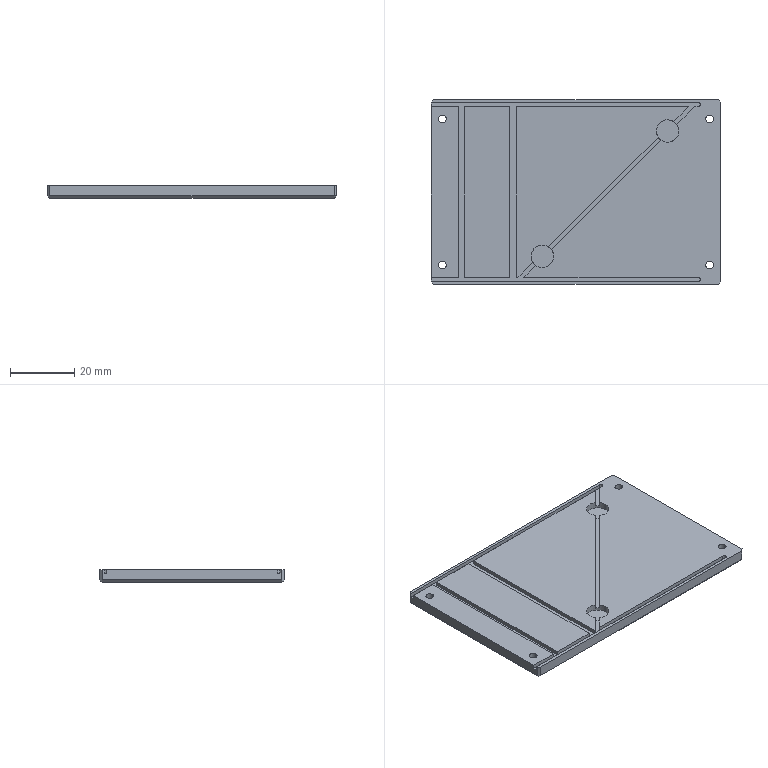Part | STEP file | ASND-0110-OPT-CO60-X-V1.0 side plate | 1 solid | 67 faces | box 90 x 57.4 x 4 mm | volume 19730 mm3 | plane 43 | cylinder 16 | cone 8 | commonest cylinder face diameters 2.4 x8 1.2 x4 7 x4